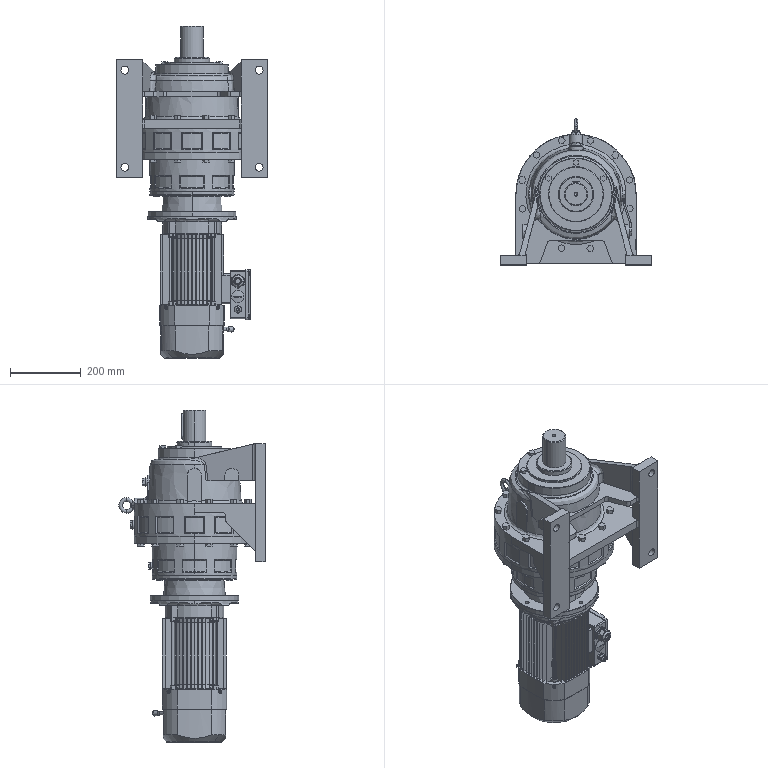Part | SolidWorks | features BaseBody 24 | 24 solids | 4524 faces | volume 37665619 mm3 | plane 3199 | spline 601 | cylinder 493 | cone 174 | torus 56 | sphere 1 | commonest cylinder face diameters 2 x71 162 x44 142 x41 6 x19 20 x19 7 x18